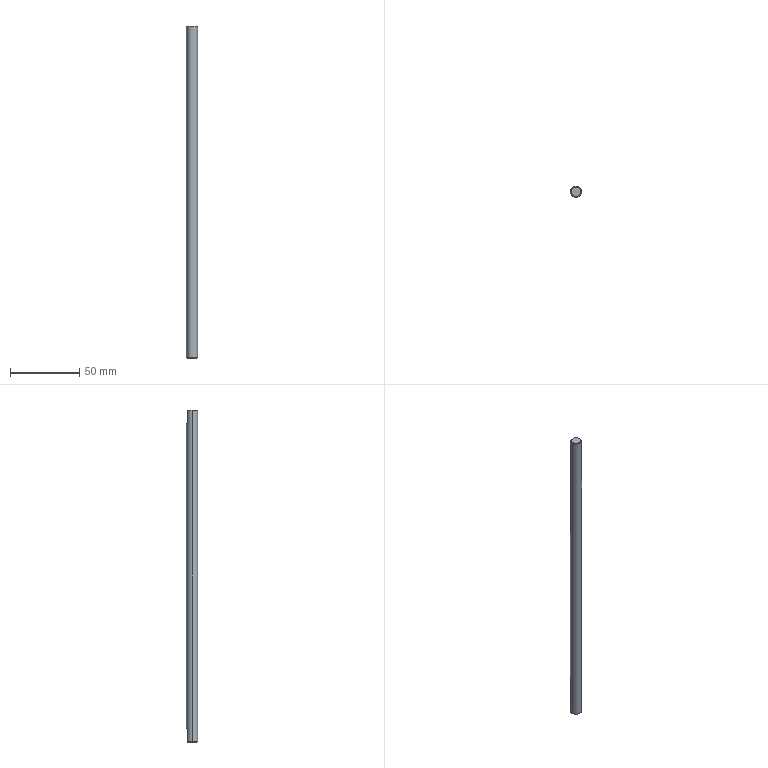Part | STEP file | CA-10-012Pusher Rod_Default | 1 solid | 14 faces | box 8 x 8 x 240 mm | volume 11986 mm3 | cone 6 | plane 6 | cylinder 2 | commonest cylinder face diameters 8 x2
STEP:
#1=CARTESIAN_POINT('',(0.,0.,0.));
#2=DIRECTION('',(0.,0.,1.));
#3=DIRECTION('',(1.,0.,0.));
#4=AXIS2_PLACEMENT_3D('',#1,#2,#3);
#5=CARTESIAN_POINT('',(3.5,0.,120.));
#6=VERTEX_POINT('',#5);
#7=CARTESIAN_POINT('',(1.803,3.,120.));
#8=VERTEX_POINT('',#7);
#9=CARTESIAN_POINT('',(0.,0.,120.));
#10=DIRECTION('',(0.,0.,1.));
#11=DIRECTION('',(1.,0.,0.));
#12=AXIS2_PLACEMENT_3D('',#9,#10,#11);
#13=CIRCLE('',#12,3.5);
#14=CARTESIAN_POINT('',(0.,0.,120.));
#15=DIRECTION('',(0.,0.,-1.));
#16=DIRECTION('',(-1.,0.,0.));
#17=AXIS2_PLACEMENT_3D('',#14,#15,#16);
#18=CONICAL_SURFACE('',#17,3.5,0.7854);
#19=CARTESIAN_POINT('',(3.142,0.));
#20=DIRECTION('',(-1.,0.));
#21=VECTOR('',#20,1.);
#22=LINE('',#19,#21);
#23=(GEOMETRIC_REPRESENTATION_CONTEXT(2)PARAMETRIC_REPRESENTATION_CONTEXT()REPRESENTATION_CONTEXT('',''));
#24=DEFINITIONAL_REPRESENTATION('',(#22),#23);
#25=PCURVE('',#18,#24);
#26=CARTESIAN_POINT('',(0.,0.,120.));
#27=DIRECTION('',(0.,0.,1.));
#28=DIRECTION('',(1.,0.,0.));
#29=AXIS2_PLACEMENT_3D('',#26,#27,#28);
#30=PLANE('',#29);
#31=CARTESIAN_POINT('',(0.,0.));
#32=DIRECTION('',(1.,0.));
#33=AXIS2_PLACEMENT_2D('',#31,#32);
#34=CIRCLE('',#33,3.5);
#35=(GEOMETRIC_REPRESENTATION_CONTEXT(2)PARAMETRIC_REPRESENTATION_CONTEXT()REPRESENTATION_CONTEXT('',''));
#36=DEFINITIONAL_REPRESENTATION('',(#34),#35);
#37=PCURVE('',#30,#36);
#38=SURFACE_CURVE('',#13,(#25,#37),.PCURVE_S1.);
#39=EDGE_CURVE('',#6,#8,#38,.T.);
#40=ORIENTED_EDGE('',*,*,#39,.F.);
#41=CARTESIAN_POINT('',(4.,0.,119.5));
#42=VERTEX_POINT('',#41);
#43=CARTESIAN_POINT('',(3.5,0.,120.));
#44=DIRECTION('',(0.7071,0.,-0.7071));
#45=VECTOR('',#44,1.);
#46=LINE('',#43,#45);
#47=CARTESIAN_POINT('',(3.142,0.));
#48=DIRECTION('',(0.,1.));
#49=VECTOR('',#48,1.);
#50=LINE('',#47,#49);
#51=(GEOMETRIC_REPRESENTATION_CONTEXT(2)PARAMETRIC_REPRESENTATION_CONTEXT()REPRESENTATION_CONTEXT('',''));
#52=DEFINITIONAL_REPRESENTATION('',(#50),#51);
#53=PCURVE('',#18,#52);
#54=CARTESIAN_POINT('',(0.,0.,120.));
#55=DIRECTION('',(0.,0.,-1.));
#56=DIRECTION('',(-1.,0.,0.));
#57=AXIS2_PLACEMENT_3D('',#54,#55,#56);
#58=CONICAL_SURFACE('',#57,3.5,0.7854);
#59=CARTESIAN_POINT('',(3.142,0.));
#60=DIRECTION('',(0.,1.));
#61=VECTOR('',#60,1.);
#62=LINE('',#59,#61);
#63=(GEOMETRIC_REPRESENTATION_CONTEXT(2)PARAMETRIC_REPRESENTATION_CONTEXT()REPRESENTATION_CONTEXT('',''));
#64=DEFINITIONAL_REPRESENTATION('',(#62),#63);
#65=PCURVE('',#58,#64);
#66=SURFACE_CURVE('',#46,(#53,#65),.PCURVE_S1.);
#67=EDGE_CURVE('',#6,#42,#66,.T.);
#68=ORIENTED_EDGE('',*,*,#67,.T.);
#69=CARTESIAN_POINT('',(2.646,3.,119.5));
#70=VERTEX_POINT('',#69);
#71=CARTESIAN_POINT('',(0.,0.,119.5));
#72=DIRECTION('',(0.,0.,-1.));
#73=DIRECTION('',(1.,0.,0.));
#74=AXIS2_PLACEMENT_3D('',#71,#72,#73);
#75=CIRCLE('',#74,4.);
#76=CARTESIAN_POINT('',(-3.142,0.5));
#77=DIRECTION('',(1.,0.));
#78=VECTOR('',#77,1.);
#79=LINE('',#76,#78);
#80=(GEOMETRIC_REPRESENTATION_CONTEXT(2)PARAMETRIC_REPRESENTATION_CONTEXT()REPRESENTATION_CONTEXT('',''));
#81=DEFINITIONAL_REPRESENTATION('',(#79),#80);
#82=PCURVE('',#18,#81);
#83=CARTESIAN_POINT('',(0.,0.,120.));
#84=DIRECTION('',(0.,0.,-1.));
#85=DIRECTION('',(-1.,0.,0.));
#86=AXIS2_PLACEMENT_3D('',#83,#84,#85);
#87=CYLINDRICAL_SURFACE('',#86,4.);
#88=CARTESIAN_POINT('',(-3.142,0.5));
#89=DIRECTION('',(1.,0.));
#90=VECTOR('',#89,1.);
#91=LINE('',#88,#90);
#92=(GEOMETRIC_REPRESENTATION_CONTEXT(2)PARAMETRIC_REPRESENTATION_CONTEXT()REPRESENTATION_CONTEXT('',''));
#93=DEFINITIONAL_REPRESENTATION('',(#91),#92);
#94=PCURVE('',#87,#93);
#95=SURFACE_CURVE('',#75,(#82,#94),.PCURVE_S1.);
#96=EDGE_CURVE('',#70,#42,#95,.T.);
#97=ORIENTED_EDGE('',*,*,#96,.F.);
#98=CARTESIAN_POINT('',(1.803,3.,120.));
#99=CARTESIAN_POINT('',(2.092,3.,119.851));
#100=CARTESIAN_POINT('',(2.373,3.,119.68));
#101=CARTESIAN_POINT('',(2.646,3.,119.5));
#102=B_SPLINE_CURVE_WITH_KNOTS('',3,(#98,#99,#100,#101),.UNSPECIFIED.,.F.,.F.,(4,4),(0.01215,0.01312),.PIECEWISE_BEZIER_KNOTS.);
#103=CARTESIAN_POINT('',(2.112,0.));
#104=CARTESIAN_POINT('',(2.115,0.006781));
#105=CARTESIAN_POINT('',(2.122,0.02043));
#106=CARTESIAN_POINT('',(2.131,0.04117));
#107=CARTESIAN_POINT('',(2.14,0.06217));
#108=CARTESIAN_POINT('',(2.15,0.08341));
#109=CARTESIAN_POINT('',(2.159,0.1049));
#110=CARTESIAN_POINT('',(2.167,0.1266));
#111=CARTESIAN_POINT('',(2.176,0.1485));
#112=CARTESIAN_POINT('',(2.185,0.1707));
#113=CARTESIAN_POINT('',(2.194,0.1931));
#114=CARTESIAN_POINT('',(2.202,0.2156));
#115=CARTESIAN_POINT('',(2.21,0.2384));
#116=CARTESIAN_POINT('',(2.218,0.2614));
#117=CARTESIAN_POINT('',(2.226,0.2845));
#118=CARTESIAN_POINT('',(2.234,0.3078));
#119=CARTESIAN_POINT('',(2.242,0.3313));
#120=CARTESIAN_POINT('',(2.25,0.355));
#121=CARTESIAN_POINT('',(2.257,0.3788));
#122=CARTESIAN_POINT('',(2.265,0.4028));
#123=CARTESIAN_POINT('',(2.272,0.4269));
#124=CARTESIAN_POINT('',(2.279,0.4511));
#125=CARTESIAN_POINT('',(2.287,0.4755));
#126=CARTESIAN_POINT('',(2.291,0.4918));
#127=CARTESIAN_POINT('',(2.294,0.5));
#128=B_SPLINE_CURVE_WITH_KNOTS('',3,(#103,#104,#105,#106,#107,#108,#109,#110,#111,#112,#113,#114,#115,#116,#117,#118,#119,#120,#121,#122,#123,#124,#125,#126,#127),.UNSPECIFIED.,.F.,.F.,(4,1,1,1,1,1,1,1,1,1,1,1,1,1,1,1,1,1,1,1,1,1,4),(0.01215,0.01219,0.01223,0.01228,0.01232,0.01237,0.01241,0.01245,0.0125,0.01254,0.01259,0.01263,0.01268,0.01272,0.01276,0.01281,0.01285,0.0129,0.01294,0.01299,0.01303,0.01307,0.01312),.QUASI_UNIFORM_KNOTS.);
#129=(GEOMETRIC_REPRESENTATION_CONTEXT(2)PARAMETRIC_REPRESENTATION_CONTEXT()REPRESENTATION_CONTEXT('',''));
#130=DEFINITIONAL_REPRESENTATION('',(#128),#129);
#131=PCURVE('',#18,#130);
#132=CARTESIAN_POINT('',(-3.991,3.,110.));
#133=DIRECTION('',(0.,-1.,0.));
#134=DIRECTION('',(0.,0.,-1.));
#135=AXIS2_PLACEMENT_3D('',#132,#133,#134);
#136=PLANE('',#135);
#137=CARTESIAN_POINT('',(-10.,5.794));
#138=CARTESIAN_POINT('',(-9.851,6.084));
#139=CARTESIAN_POINT('',(-9.68,6.365));
#140=CARTESIAN_POINT('',(-9.5,6.637));
#141=B_SPLINE_CURVE_WITH_KNOTS('',3,(#137,#138,#139,#140),.UNSPECIFIED.,.F.,.F.,(4,4),(0.01215,0.01312),.PIECEWISE_BEZIER_KNOTS.);
#142=(GEOMETRIC_REPRESENTATION_CONTEXT(2)PARAMETRIC_REPRESENTATION_CONTEXT()REPRESENTATION_CONTEXT('',''));
#143=DEFINITIONAL_REPRESENTATION('',(#141),#142);
#144=PCURVE('',#136,#143);
#145=SURFACE_CURVE('',#102,(#131,#144),.PCURVE_S1.);
#146=EDGE_CURVE('',#8,#70,#145,.T.);
#147=ORIENTED_EDGE('',*,*,#146,.F.);
#148=EDGE_LOOP('',(#40,#68,#97,#147));
#149=FACE_BOUND('',#148,.T.);
#150=ADVANCED_FACE('',(#149),#18,.T.);
#151=ORIENTED_EDGE('',*,*,#67,.F.);
#152=CARTESIAN_POINT('',(-3.5,0.,120.));
#153=VERTEX_POINT('',#152);
#154=CARTESIAN_POINT('',(0.,0.,120.));
#155=DIRECTION('',(0.,0.,1.));
#156=DIRECTION('',(1.,0.,0.));
#157=AXIS2_PLACEMENT_3D('',#154,#155,#156);
#158=CIRCLE('',#157,3.5);
#159=CARTESIAN_POINT('',(9.425,0.));
#160=DIRECTION('',(-1.,0.));
#161=VECTOR('',#160,1.);
#162=LINE('',#159,#161);
#163=(GEOMETRIC_REPRESENTATION_CONTEXT(2)PARAMETRIC_REPRESENTATION_CONTEXT()REPRESENTATION_CONTEXT('',''));
#164=DEFINITIONAL_REPRESENTATION('',(#162),#163);
#165=PCURVE('',#58,#164);
#166=CARTESIAN_POINT('',(0.,0.));
#167=DIRECTION('',(1.,0.));
#168=AXIS2_PLACEMENT_2D('',#166,#167);
#169=CIRCLE('',#168,3.5);
#170=(GEOMETRIC_REPRESENTATION_CONTEXT(2)PARAMETRIC_REPRESENTATION_CONTEXT()REPRESENTATION_CONTEXT('',''));
#171=DEFINITIONAL_REPRESENTATION('',(#169),#170);
#172=PCURVE('',#30,#171);
#173=SURFACE_CURVE('',#158,(#165,#172),.PCURVE_S1.);
#174=EDGE_CURVE('',#153,#6,#173,.T.);
#175=ORIENTED_EDGE('',*,*,#174,.F.);
#176=CARTESIAN_POINT('',(-4.,0.,119.5));
#177=VERTEX_POINT('',#176);
#178=CARTESIAN_POINT('',(-3.5,0.,120.));
#179=DIRECTION('',(-0.7071,0.,-0.7071));
#180=VECTOR('',#179,1.);
#181=LINE('',#178,#180);
#182=CARTESIAN_POINT('',(6.283,0.));
#183=DIRECTION('',(0.,1.));
#184=VECTOR('',#183,1.);
#185=LINE('',#182,#184);
#186=(GEOMETRIC_REPRESENTATION_CONTEXT(2)PARAMETRIC_REPRESENTATION_CONTEXT()REPRESENTATION_CONTEXT('',''));
#187=DEFINITIONAL_REPRESENTATION('',(#185),#186);
#188=PCURVE('',#58,#187);
#189=CARTESIAN_POINT('',(0.,0.,120.));
#190=DIRECTION('',(0.,0.,-1.));
#191=DIRECTION('',(-1.,0.,0.));
#192=AXIS2_PLACEMENT_3D('',#189,#190,#191);
#193=CONICAL_SURFACE('',#192,3.5,0.7854);
#194=CARTESIAN_POINT('',(0.,0.));
#195=DIRECTION('',(0.,1.));
#196=VECTOR('',#195,1.);
#197=LINE('',#194,#196);
#198=(GEOMETRIC_REPRESENTATION_CONTEXT(2)PARAMETRIC_REPRESENTATION_CONTEXT()REPRESENTATION_CONTEXT('',''));
#199=DEFINITIONAL_REPRESENTATION('',(#197),#198);
#200=PCURVE('',#193,#199);
#201=SURFACE_CURVE('',#181,(#188,#200),.PCURVE_S1.);
#202=EDGE_CURVE('',#153,#177,#201,.T.);
#203=ORIENTED_EDGE('',*,*,#202,.T.);
#204=CARTESIAN_POINT('',(0.,0.,119.5));
#205=DIRECTION('',(0.,0.,-1.));
#206=DIRECTION('',(1.,0.,0.));
#207=AXIS2_PLACEMENT_3D('',#204,#205,#206);
#208=CIRCLE('',#207,4.);
#209=CARTESIAN_POINT('',(3.142,0.5));
#210=DIRECTION('',(1.,0.));
#211=VECTOR('',#210,1.);
#212=LINE('',#209,#211);
#213=(GEOMETRIC_REPRESENTATION_CONTEXT(2)PARAMETRIC_REPRESENTATION_CONTEXT()REPRESENTATION_CONTEXT('',''));
#214=DEFINITIONAL_REPRESENTATION('',(#212),#213);
#215=PCURVE('',#58,#214);
#216=CARTESIAN_POINT('',(0.,0.,120.));
#217=DIRECTION('',(0.,0.,-1.));
#218=DIRECTION('',(-1.,0.,0.));
#219=AXIS2_PLACEMENT_3D('',#216,#217,#218);
#220=CYLINDRICAL_SURFACE('',#219,4.);
#221=CARTESIAN_POINT('',(3.142,0.5));
#222=DIRECTION('',(1.,0.));
#223=VECTOR('',#222,1.);
#224=LINE('',#221,#223);
#225=(GEOMETRIC_REPRESENTATION_CONTEXT(2)PARAMETRIC_REPRESENTATION_CONTEXT()REPRESENTATION_CONTEXT('',''));
#226=DEFINITIONAL_REPRESENTATION('',(#224),#225);
#227=PCURVE('',#220,#226);
#228=SURFACE_CURVE('',#208,(#215,#227),.PCURVE_S1.);
#229=EDGE_CURVE('',#42,#177,#228,.T.);
#230=ORIENTED_EDGE('',*,*,#229,.F.);
#231=EDGE_LOOP('',(#151,#175,#203,#230));
#232=FACE_BOUND('',#231,.T.);
#233=ADVANCED_FACE('',(#232),#58,.T.);
#234=CARTESIAN_POINT('',(-3.5,0.,-120.));
#235=VERTEX_POINT('',#234);
#236=CARTESIAN_POINT('',(-1.803,3.,-120.));
#237=VERTEX_POINT('',#236);
#238=CARTESIAN_POINT('',(0.,0.,-120.));
#239=DIRECTION('',(0.,0.,-1.));
#240=DIRECTION('',(1.,0.,0.));
#241=AXIS2_PLACEMENT_3D('',#238,#239,#240);
#242=CIRCLE('',#241,3.5);
#243=CARTESIAN_POINT('',(0.,0.,-119.5));
#244=DIRECTION('',(0.,0.,1.));
#245=DIRECTION('',(1.,0.,0.));
#246=AXIS2_PLACEMENT_3D('',#243,#244,#245);
#247=CONICAL_SURFACE('',#246,4.,0.7854);
#248=CARTESIAN_POINT('',(6.283,-0.5));
#249=DIRECTION('',(-1.,0.));
#250=VECTOR('',#249,1.);
#251=LINE('',#248,#250);
#252=(GEOMETRIC_REPRESENTATION_CONTEXT(2)PARAMETRIC_REPRESENTATION_CONTEXT()REPRESENTATION_CONTEXT('',''));
#253=DEFINITIONAL_REPRESENTATION('',(#251),#252);
#254=PCURVE('',#247,#253);
#255=CARTESIAN_POINT('',(0.,0.,-120.));
#256=DIRECTION('',(0.,0.,1.));
#257=DIRECTION('',(1.,0.,0.));
#258=AXIS2_PLACEMENT_3D('',#255,#256,#257);
#259=PLANE('',#258);
#260=CARTESIAN_POINT('',(3.5,0.));
#261=CARTESIAN_POINT('',(3.5,-6.062));
#262=CARTESIAN_POINT('',(-1.75,-3.031));
#263=CARTESIAN_POINT('',(-7.,0.));
#264=CARTESIAN_POINT('',(-1.75,3.031));
#265=CARTESIAN_POINT('',(3.5,6.062));
#266=CARTESIAN_POINT('',(3.5,0.));
#267=(BOUNDED_CURVE()B_SPLINE_CURVE(2,(#260,#261,#262,#263,#264,#265,#266),.UNSPECIFIED.,.T.,.F.)B_SPLINE_CURVE_WITH_KNOTS((1,2,2,2,2,1),(-2.094,0.,2.094,4.189,6.283,8.378),.UNSPECIFIED.)CURVE()GEOMETRIC_REPRESENTATION_ITEM()RATIONAL_B_SPLINE_CURVE((1.,0.5,1.,0.5,1.,0.5,1.))REPRESENTATION_ITEM(''));
#268=(GEOMETRIC_REPRESENTATION_CONTEXT(2)PARAMETRIC_REPRESENTATION_CONTEXT()REPRESENTATION_CONTEXT('',''));
#269=DEFINITIONAL_REPRESENTATION('',(#267),#268);
#270=PCURVE('',#259,#269);
#271=SURFACE_CURVE('',#242,(#254,#270),.PCURVE_S1.);
#272=EDGE_CURVE('',#235,#237,#271,.T.);
#273=ORIENTED_EDGE('',*,*,#272,.F.);
#274=CARTESIAN_POINT('',(-4.,0.,-119.5));
#275=VERTEX_POINT('',#274);
#276=CARTESIAN_POINT('',(-4.,0.,-119.5));
#277=DIRECTION('',(-0.7071,0.,0.7071));
#278=VECTOR('',#277,1.);
#279=LINE('',#276,#278);
#280=CARTESIAN_POINT('',(3.142,0.));
#281=DIRECTION('',(0.,1.));
#282=VECTOR('',#281,1.);
#283=LINE('',#280,#282);
#284=(GEOMETRIC_REPRESENTATION_CONTEXT(2)PARAMETRIC_REPRESENTATION_CONTEXT()REPRESENTATION_CONTEXT('',''));
#285=DEFINITIONAL_REPRESENTATION('',(#283),#284);
#286=PCURVE('',#247,#285);
#287=CARTESIAN_POINT('',(0.,0.,-119.5));
#288=DIRECTION('',(0.,0.,1.));
#289=DIRECTION('',(1.,0.,0.));
#290=AXIS2_PLACEMENT_3D('',#287,#288,#289);
#291=CONICAL_SURFACE('',#290,4.,0.7854);
#292=CARTESIAN_POINT('',(3.142,0.));
#293=DIRECTION('',(0.,1.));
#294=VECTOR('',#293,1.);
#295=LINE('',#292,#294);
#296=(GEOMETRIC_REPRESENTATION_CONTEXT(2)PARAMETRIC_REPRESENTATION_CONTEXT()REPRESENTATION_CONTEXT('',''));
#297=DEFINITIONAL_REPRESENTATION('',(#295),#296);
#298=PCURVE('',#291,#297);
#299=SURFACE_CURVE('',#279,(#286,#298),.PCURVE_S1.);
#300=EDGE_CURVE('',#235,#275,#299,.T.);
#301=ORIENTED_EDGE('',*,*,#300,.T.);
#302=CARTESIAN_POINT('',(-2.646,3.,-119.5));
#303=VERTEX_POINT('',#302);
#304=CARTESIAN_POINT('',(0.,0.,-119.5));
#305=DIRECTION('',(0.,0.,1.));
#306=DIRECTION('',(1.,0.,0.));
#307=AXIS2_PLACEMENT_3D('',#304,#305,#306);
#308=CIRCLE('',#307,4.);
#309=CARTESIAN_POINT('',(0.,0.));
#310=DIRECTION('',(1.,0.));
#311=VECTOR('',#310,1.);
#312=LINE('',#309,#311);
#313=(GEOMETRIC_REPRESENTATION_CONTEXT(2)PARAMETRIC_REPRESENTATION_CONTEXT()REPRESENTATION_CONTEXT('',''));
#314=DEFINITIONAL_REPRESENTATION('',(#312),#313);
#315=PCURVE('',#247,#314);
#316=CARTESIAN_POINT('',(3.142,239.5));
#317=DIRECTION('',(-1.,0.));
#318=VECTOR('',#317,1.);
#319=LINE('',#316,#318);
#320=(GEOMETRIC_REPRESENTATION_CONTEXT(2)PARAMETRIC_REPRESENTATION_CONTEXT()REPRESENTATION_CONTEXT('',''));
#321=DEFINITIONAL_REPRESENTATION('',(#319),#320);
#322=PCURVE('',#87,#321);
#323=SURFACE_CURVE('',#308,(#315,#322),.PCURVE_S1.);
#324=EDGE_CURVE('',#303,#275,#323,.T.);
#325=ORIENTED_EDGE('',*,*,#324,.F.);
#326=CARTESIAN_POINT('',(-2.646,3.,-119.5));
#327=CARTESIAN_POINT('',(-2.374,3.,-119.68));
#328=CARTESIAN_POINT('',(-2.095,3.,-119.849));
#329=CARTESIAN_POINT('',(-1.803,3.,-120.));
#330=B_SPLINE_CURVE_WITH_KNOTS('',3,(#326,#327,#328,#329),.UNSPECIFIED.,.F.,.F.,(4,4),(0.007417,0.008397),.PIECEWISE_BEZIER_KNOTS.);
#331=CARTESIAN_POINT('',(2.294,0.));
#332=CARTESIAN_POINT('',(2.291,-0.008169));
#333=CARTESIAN_POINT('',(2.287,-0.02446));
#334=CARTESIAN_POINT('',(2.279,-0.04877));
#335=CARTESIAN_POINT('',(2.272,-0.07295));
#336=CARTESIAN_POINT('',(2.265,-0.09698));
#337=CARTESIAN_POINT('',(2.257,-0.1209));
#338=CARTESIAN_POINT('',(2.25,-0.1446));
#339=CARTESIAN_POINT('',(2.242,-0.1682));
#340=CARTESIAN_POINT('',(2.235,-0.1916));
#341=CARTESIAN_POINT('',(2.227,-0.2149));
#342=CARTESIAN_POINT('',(2.219,-0.238));
#343=CARTESIAN_POINT('',(2.21,-0.2609));
#344=CARTESIAN_POINT('',(2.202,-0.2836));
#345=CARTESIAN_POINT('',(2.194,-0.3062));
#346=CARTESIAN_POINT('',(2.185,-0.3285));
#347=CARTESIAN_POINT('',(2.177,-0.3507));
#348=CARTESIAN_POINT('',(2.168,-0.3727));
#349=CARTESIAN_POINT('',(2.159,-0.3945));
#350=CARTESIAN_POINT('',(2.15,-0.416));
#351=CARTESIAN_POINT('',(2.141,-0.4374));
#352=CARTESIAN_POINT('',(2.131,-0.4585));
#353=CARTESIAN_POINT('',(2.122,-0.4794));
#354=CARTESIAN_POINT('',(2.115,-0.4932));
#355=CARTESIAN_POINT('',(2.112,-0.5));
#356=B_SPLINE_CURVE_WITH_KNOTS('',3,(#331,#332,#333,#334,#335,#336,#337,#338,#339,#340,#341,#342,#343,#344,#345,#346,#347,#348,#349,#350,#351,#352,#353,#354,#355),.UNSPECIFIED.,.F.,.F.,(4,1,1,1,1,1,1,1,1,1,1,1,1,1,1,1,1,1,1,1,1,1,4),(0.007417,0.007461,0.007506,0.007551,0.007595,0.00764,0.007684,0.007729,0.007773,0.007818,0.007863,0.007907,0.007952,0.007996,0.008041,0.008085,0.00813,0.008175,0.008219,0.008264,0.008308,0.008353,0.008397),.QUASI_UNIFORM_KNOTS.);
#357=(GEOMETRIC_REPRESENTATION_CONTEXT(2)PARAMETRIC_REPRESENTATION_CONTEXT()REPRESENTATION_CONTEXT('',''));
#358=DEFINITIONAL_REPRESENTATION('',(#356),#357);
#359=PCURVE('',#247,#358);
#360=CARTESIAN_POINT('',(-3.991,3.,-110.));
#361=DIRECTION('',(0.,1.,0.));
#362=DIRECTION('',(0.,0.,1.));
#363=AXIS2_PLACEMENT_3D('',#360,#361,#362);
#364=PLANE('',#363);
#365=CARTESIAN_POINT('',(-9.5,1.346));
#366=CARTESIAN_POINT('',(-9.68,1.617));
#367=CARTESIAN_POINT('',(-9.849,1.896));
#368=CARTESIAN_POINT('',(-10.,2.189));
#369=B_SPLINE_CURVE_WITH_KNOTS('',3,(#365,#366,#367,#368),.UNSPECIFIED.,.F.,.F.,(4,4),(0.007417,0.008397),.PIECEWISE_BEZIER_KNOTS.);
#370=(GEOMETRIC_REPRESENTATION_CONTEXT(2)PARAMETRIC_REPRESENTATION_CONTEXT()REPRESENTATION_CONTEXT('',''));
#371=DEFINITIONAL_REPRESENTATION('',(#369),#370);
#372=PCURVE('',#364,#371);
#373=SURFACE_CURVE('',#330,(#359,#372),.PCURVE_S1.);
#374=EDGE_CURVE('',#303,#237,#373,.T.);
#375=ORIENTED_EDGE('',*,*,#374,.T.);
#376=EDGE_LOOP('',(#273,#301,#325,#375));
#377=FACE_BOUND('',#376,.T.);
#378=ADVANCED_FACE('',(#377),#247,.T.);
#379=ORIENTED_EDGE('',*,*,#300,.F.);
#380=CARTESIAN_POINT('',(3.5,0.,-120.));
#381=VERTEX_POINT('',#380);
#382=CARTESIAN_POINT('',(0.,0.,-120.));
#383=DIRECTION('',(0.,0.,-1.));
#384=DIRECTION('',(1.,0.,0.));
#385=AXIS2_PLACEMENT_3D('',#382,#383,#384);
#386=CIRCLE('',#385,3.5);
#387=CARTESIAN_POINT('',(6.283,-0.5));
#388=DIRECTION('',(-1.,0.));
#389=VECTOR('',#388,1.);
#390=LINE('',#387,#389);
#391=(GEOMETRIC_REPRESENTATION_CONTEXT(2)PARAMETRIC_REPRESENTATION_CONTEXT()REPRESENTATION_CONTEXT('',''));
#392=DEFINITIONAL_REPRESENTATION('',(#390),#391);
#393=PCURVE('',#291,#392);
#394=CARTESIAN_POINT('',(3.5,0.));
#395=CARTESIAN_POINT('',(3.5,-6.062));
#396=CARTESIAN_POINT('',(-1.75,-3.031));
#397=CARTESIAN_POINT('',(-7.,0.));
#398=CARTESIAN_POINT('',(-1.75,3.031));
#399=CARTESIAN_POINT('',(3.5,6.062));
#400=CARTESIAN_POINT('',(3.5,0.));
#401=(BOUNDED_CURVE()B_SPLINE_CURVE(2,(#394,#395,#396,#397,#398,#399,#400),.UNSPECIFIED.,.T.,.F.)B_SPLINE_CURVE_WITH_KNOTS((1,2,2,2,2,1),(-2.094,0.,2.094,4.189,6.283,8.378),.UNSPECIFIED.)CURVE()GEOMETRIC_REPRESENTATION_ITEM()RATIONAL_B_SPLINE_CURVE((1.,0.5,1.,0.5,1.,0.5,1.))REPRESENTATION_ITEM(''));
#402=(GEOMETRIC_REPRESENTATION_CONTEXT(2)PARAMETRIC_REPRESENTATION_CONTEXT()REPRESENTATION_CONTEXT('',''));
#403=DEFINITIONAL_REPRESENTATION('',(#401),#402);
#404=PCURVE('',#259,#403);
#405=SURFACE_CURVE('',#386,(#393,#404),.PCURVE_S1.);
#406=EDGE_CURVE('',#381,#235,#405,.T.);
#407=ORIENTED_EDGE('',*,*,#406,.F.);
#408=CARTESIAN_POINT('',(4.,0.,-119.5));
#409=VERTEX_POINT('',#408);
#410=CARTESIAN_POINT('',(4.,0.,-119.5));
#411=DIRECTION('',(0.7071,0.,0.7071));
#412=VECTOR('',#411,1.);
#413=LINE('',#410,#412);
#414=CARTESIAN_POINT('',(6.283,0.));
#415=DIRECTION('',(0.,1.));
#416=VECTOR('',#415,1.);
#417=LINE('',#414,#416);
#418=(GEOMETRIC_REPRESENTATION_CONTEXT(2)PARAMETRIC_REPRESENTATION_CONTEXT()REPRESENTATION_CONTEXT('',''));
#419=DEFINITIONAL_REPRESENTATION('',(#417),#418);
#420=PCURVE('',#291,#419);
#421=CARTESIAN_POINT('',(0.,0.,-119.5));
#422=DIRECTION('',(0.,0.,1.));
#423=DIRECTION('',(1.,0.,0.));
#424=AXIS2_PLACEMENT_3D('',#421,#422,#423);
#425=CONICAL_SURFACE('',#424,4.,0.7854);
#426=CARTESIAN_POINT('',(0.,0.));
#427=DIRECTION('',(0.,1.));
#428=VECTOR('',#427,1.);
#429=LINE('',#426,#428);
#430=(GEOMETRIC_REPRESENTATION_CONTEXT(2)PARAMETRIC_REPRESENTATION_CONTEXT()REPRESENTATION_CONTEXT('',''));
#431=DEFINITIONAL_REPRESENTATION('',(#429),#430);
#432=PCURVE('',#425,#431);
#433=SURFACE_CURVE('',#413,(#420,#432),.PCURVE_S1.);
#434=EDGE_CURVE('',#381,#409,#433,.T.);
#435=ORIENTED_EDGE('',*,*,#434,.T.);
#436=CARTESIAN_POINT('',(0.,0.,-119.5));
#437=DIRECTION('',(0.,0.,1.));
#438=DIRECTION('',(1.,0.,0.));
#439=AXIS2_PLACEMENT_3D('',#436,#437,#438);
#440=CIRCLE('',#439,4.);
#441=CARTESIAN_POINT('',(0.,0.));
#442=DIRECTION('',(1.,0.));
#443=VECTOR('',#442,1.);
#444=LINE('',#441,#443);
#445=(GEOMETRIC_REPRESENTATION_CONTEXT(2)PARAMETRIC_REPRESENTATION_CONTEXT()REPRESENTATION_CONTEXT('',''));
#446=DEFINITIONAL_REPRESENTATION('',(#444),#445);
#447=PCURVE('',#291,#446);
#448=CARTESIAN_POINT('',(9.425,239.5));
#449=DIRECTION('',(-1.,0.));
#450=VECTOR('',#449,1.);
#451=LINE('',#448,#450);
#452=(GEOMETRIC_REPRESENTATION_CONTEXT(2)PARAMETRIC_REPRESENTATION_CONTEXT()REPRESENTATION_CONTEXT('',''));
#453=DEFINITIONAL_REPRESENTATION('',(#451),#452);
#454=PCURVE('',#220,#453);
#455=SURFACE_CURVE('',#440,(#447,#454),.PCURVE_S1.);
#456=EDGE_CURVE('',#275,#409,#455,.T.);
#457=ORIENTED_EDGE('',*,*,#456,.F.);
#458=EDGE_LOOP('',(#379,#407,#435,#457));
#459=FACE_BOUND('',#458,.T.);
#460=ADVANCED_FACE('',(#459),#291,.T.);
#461=ORIENTED_EDGE('',*,*,#96,.T.);
#462=CARTESIAN_POINT('',(4.,0.,120.));
#463=DIRECTION('',(0.,0.,-1.));
#464=VECTOR('',#463,1.);
#465=LINE('',#462,#464);
#466=CARTESIAN_POINT('',(3.142,0.));
#467=DIRECTION('',(0.,1.));
#468=VECTOR('',#467,1.);
#469=LINE('',#466,#468);
#470=(GEOMETRIC_REPRESENTATION_CONTEXT(2)PARAMETRIC_REPRESENTATION_CONTEXT()REPRESENTATION_CONTEXT('',''));
#471=DEFINITIONAL_REPRESENTATION('',(#469),#470);
#472=PCURVE('',#87,#471);
#473=CARTESIAN_POINT('',(3.142,0.));
#474=DIRECTION('',(0.,1.));
#475=VECTOR('',#474,1.);
#476=LINE('',#473,#475);
#477=(GEOMETRIC_REPRESENTATION_CONTEXT(2)PARAMETRIC_REPRESENTATION_CONTEXT()REPRESENTATION_CONTEXT('',''));
#478=DEFINITIONAL_REPRESENTATION('',(#476),#477);
#479=PCURVE('',#220,#478);
#480=SURFACE_CURVE('',#465,(#472,#479),.PCURVE_S1.);
#481=EDGE_CURVE('',#42,#409,#480,.T.);
#482=ORIENTED_EDGE('',*,*,#481,.T.);
#483=CARTESIAN_POINT('',(2.646,3.,-119.5));
#484=VERTEX_POINT('',#483);
#485=CARTESIAN_POINT('',(0.,0.,-119.5));
#486=DIRECTION('',(0.,0.,1.));
#487=DIRECTION('',(1.,0.,0.));
#488=AXIS2_PLACEMENT_3D('',#485,#486,#487);
#489=CIRCLE('',#488,4.);
#490=CARTESIAN_POINT('',(3.142,239.5));
#491=DIRECTION('',(-1.,0.));
#492=VECTOR('',#491,1.);
#493=LINE('',#490,#492);
#494=(GEOMETRIC_REPRESENTATION_CONTEXT(2)PARAMETRIC_REPRESENTATION_CONTEXT()REPRESENTATION_CONTEXT('',''));
#495=DEFINITIONAL_REPRESENTATION('',(#493),#494);
#496=PCURVE('',#87,#495);
#497=CARTESIAN_POINT('',(0.,0.));
#498=DIRECTION('',(1.,0.));
#499=VECTOR('',#498,1.);
#500=LINE('',#497,#499);
#501=(GEOMETRIC_REPRESENTATION_CONTEXT(2)PARAMETRIC_REPRESENTATION_CONTEXT()REPRESENTATION_CONTEXT('',''));
#502=DEFINITIONAL_REPRESENTATION('',(#500),#501);
#503=PCURVE('',#425,#502);
#504=SURFACE_CURVE('',#489,(#496,#503),.PCURVE_S1.);
#505=EDGE_CURVE('',#409,#484,#504,.T.);
#506=ORIENTED_EDGE('',*,*,#505,.T.);
#507=CARTESIAN_POINT('',(2.646,3.,-110.));
#508=VERTEX_POINT('',#507);
#509=CARTESIAN_POINT('',(2.646,3.,120.));
#510=DIRECTION('',(0.,0.,-1.));
#511=VECTOR('',#510,1.);
#512=LINE('',#509,#511);
#513=CARTESIAN_POINT('',(2.294,0.));
#514=DIRECTION('',(0.,1.));
#515=VECTOR('',#514,1.);
#516=LINE('',#513,#515);
#517=(GEOMETRIC_REPRESENTATION_CONTEXT(2)PARAMETRIC_REPRESENTATION_CONTEXT()REPRESENTATION_CONTEXT('',''));
#518=DEFINITIONAL_REPRESENTATION('',(#516),#517);
#519=PCURVE('',#87,#518);
#520=CARTESIAN_POINT('',(230.,6.637));
#521=DIRECTION('',(-1.,0.));
#522=VECTOR('',#521,1.);
#523=LINE('',#520,#522);
#524=(GEOMETRIC_REPRESENTATION_CONTEXT(2)PARAMETRIC_REPRESENTATION_CONTEXT()REPRESENTATION_CONTEXT('',''));
#525=DEFINITIONAL_REPRESENTATION('',(#523),#524);
#526=PCURVE('',#364,#525);
#527=SURFACE_CURVE('',#512,(#519,#526),.PCURVE_S1.);
#528=EDGE_CURVE('',#508,#484,#527,.T.);
#529=ORIENTED_EDGE('',*,*,#528,.F.);
#530=CARTESIAN_POINT('',(-2.646,3.,-110.));
#531=VERTEX_POINT('',#530);
#532=CARTESIAN_POINT('',(0.,0.,-110.));
#533=DIRECTION('',(0.,0.,-1.));
#534=DIRECTION('',(-1.,0.,0.));
#535=AXIS2_PLACEMENT_3D('',#532,#533,#534);
#536=CIRCLE('',#535,4.);
#537=CARTESIAN_POINT('',(0.,230.));
#538=DIRECTION('',(1.,0.));
#539=VECTOR('',#538,1.);
#540=LINE('',#537,#539);
#541=(GEOMETRIC_REPRESENTATION_CONTEXT(2)PARAMETRIC_REPRESENTATION_CONTEXT()REPRESENTATION_CONTEXT('',''));
#542=DEFINITIONAL_REPRESENTATION('',(#540),#541);
#543=PCURVE('',#87,#542);
#544=CARTESIAN_POINT('',(0.,0.,-110.));
#545=DIRECTION('',(0.,0.,-1.));
#546=DIRECTION('',(1.,0.,0.));
#547=AXIS2_PLACEMENT_3D('',#544,#545,#546);
#548=PLANE('',#547);
#549=CARTESIAN_POINT('',(0.,0.));
#550=DIRECTION('',(-1.,0.));
#551=AXIS2_PLACEMENT_2D('',#549,#550);
#552=CIRCLE('',#551,4.);
#553=(GEOMETRIC_REPRESENTATION_CONTEXT(2)PARAMETRIC_REPRESENTATION_CONTEXT()REPRESENTATION_CONTEXT('',''));
#554=DEFINITIONAL_REPRESENTATION('',(#552),#553);
#555=PCURVE('',#548,#554);
#556=SURFACE_CURVE('',#536,(#543,#555),.PCURVE_S1.);
#557=EDGE_CURVE('',#531,#508,#556,.T.);
#558=ORIENTED_EDGE('',*,*,#557,.F.);
#559=CARTESIAN_POINT('',(-2.646,3.,120.));
#560=DIRECTION('',(0.,0.,1.));
#561=VECTOR('',#560,1.);
#562=LINE('',#559,#561);
#563=CARTESIAN_POINT('',(0.8481,0.));
#564=DIRECTION('',(0.,-1.));
#565=VECTOR('',#564,1.);
#566=LINE('',#563,#565);
#567=(GEOMETRIC_REPRESENTATION_CONTEXT(2)PARAMETRIC_REPRESENTATION_CONTEXT()REPRESENTATION_CONTEXT('',''));
#568=DEFINITIONAL_REPRESENTATION('',(#566),#567);
#569=PCURVE('',#87,#568);
#570=CARTESIAN_POINT('',(230.,1.346));
#571=DIRECTION('',(1.,0.));
#572=VECTOR('',#571,1.);
#573=LINE('',#570,#572);
#574=(GEOMETRIC_REPRESENTATION_CONTEXT(2)PARAMETRIC_REPRESENTATION_CONTEXT()REPRESENTATION_CONTEXT('',''));
#575=DEFINITIONAL_REPRESENTATION('',(#573),#574);
#576=PCURVE('',#364,#575);
#577=SURFACE_CURVE('',#562,(#569,#576),.PCURVE_S1.);
#578=EDGE_CURVE('',#303,#531,#577,.T.);
#579=ORIENTED_EDGE('',*,*,#578,.F.);
#580=ORIENTED_EDGE('',*,*,#324,.T.);
#581=CARTESIAN_POINT('',(-4.,0.,120.));
#582=DIRECTION('',(0.,0.,-1.));
#583=VECTOR('',#582,1.);
#584=LINE('',#581,#583);
#585=CARTESIAN_POINT('',(0.,0.));
#586=DIRECTION('',(0.,1.));
#587=VECTOR('',#586,1.);
#588=LINE('',#585,#587);
#589=(GEOMETRIC_REPRESENTATION_CONTEXT(2)PARAMETRIC_REPRESENTATION_CONTEXT()REPRESENTATION_CONTEXT('',''));
#590=DEFINITIONAL_REPRESENTATION('',(#588),#589);
#591=PCURVE('',#87,#590);
#592=CARTESIAN_POINT('',(6.283,0.));
#593=DIRECTION('',(0.,1.));
#594=VECTOR('',#593,1.);
#595=LINE('',#592,#594);
#596=(GEOMETRIC_REPRESENTATION_CONTEXT(2)PARAMETRIC_REPRESENTATION_CONTEXT()REPRESENTATION_CONTEXT('',''));
#597=DEFINITIONAL_REPRESENTATION('',(#595),#596);
#598=PCURVE('',#220,#597);
#599=SURFACE_CURVE('',#584,(#591,#598),.PCURVE_S1.);
#600=EDGE_CURVE('',#177,#275,#599,.T.);
#601=ORIENTED_EDGE('',*,*,#600,.F.);
#602=CARTESIAN_POINT('',(-2.646,3.,119.5));
#603=VERTEX_POINT('',#602);
#604=CARTESIAN_POINT('',(0.,0.,119.5));
#605=DIRECTION('',(0.,0.,-1.));
#606=DIRECTION('',(1.,0.,0.));
#607=AXIS2_PLACEMENT_3D('',#604,#605,#606);
#608=CIRCLE('',#607,4.);
#609=CARTESIAN_POINT('',(-3.142,0.5));
#610=DIRECTION('',(1.,0.));
#611=VECTOR('',#610,1.);
#612=LINE('',#609,#611);
#613=(GEOMETRIC_REPRESENTATION_CONTEXT(2)PARAMETRIC_REPRESENTATION_CONTEXT()REPRESENTATION_CONTEXT('',''));
#614=DEFINITIONAL_REPRESENTATION('',(#612),#613);
#615=PCURVE('',#87,#614);
#616=CARTESIAN_POINT('',(-3.142,0.5));
#617=DIRECTION('',(1.,0.));
#618=VECTOR('',#617,1.);
#619=LINE('',#616,#618);
#620=(GEOMETRIC_REPRESENTATION_CONTEXT(2)PARAMETRIC_REPRESENTATION_CONTEXT()REPRESENTATION_CONTEXT('',''));
#621=DEFINITIONAL_REPRESENTATION('',(#619),#620);
#622=PCURVE('',#193,#621);
#623=SURFACE_CURVE('',#608,(#615,#622),.PCURVE_S1.);
#624=EDGE_CURVE('',#177,#603,#623,.T.);
#625=ORIENTED_EDGE('',*,*,#624,.T.);
#626=CARTESIAN_POINT('',(-2.646,3.,110.));
#627=VERTEX_POINT('',#626);
#628=CARTESIAN_POINT('',(-2.646,3.,120.));
#629=DIRECTION('',(0.,0.,-1.));
#630=VECTOR('',#629,1.);
#631=LINE('',#628,#630);
#632=CARTESIAN_POINT('',(0.8481,0.));
#633=DIRECTION('',(0.,1.));
#634=VECTOR('',#633,1.);
#635=LINE('',#632,#634);
#636=(GEOMETRIC_REPRESENTATION_CONTEXT(2)PARAMETRIC_REPRESENTATION_CONTEXT()REPRESENTATION_CONTEXT('',''));
#637=DEFINITIONAL_REPRESENTATION('',(#635),#636);
#638=PCURVE('',#87,#637);
#639=CARTESIAN_POINT('',(-10.,1.346));
#640=DIRECTION('',(1.,0.));
#641=VECTOR('',#640,1.);
#642=LINE('',#639,#641);
#643=(GEOMETRIC_REPRESENTATION_CONTEXT(2)PARAMETRIC_REPRESENTATION_CONTEXT()REPRESENTATION_CONTEXT('',''));
#644=DEFINITIONAL_REPRESENTATION('',(#642),#643);
#645=PCURVE('',#136,#644);
#646=SURFACE_CURVE('',#631,(#638,#645),.PCURVE_S1.);
#647=EDGE_CURVE('',#603,#627,#646,.T.);
#648=ORIENTED_EDGE('',*,*,#647,.T.);
#649=CARTESIAN_POINT('',(2.646,3.,110.));
#650=VERTEX_POINT('',#649);
#651=CARTESIAN_POINT('',(0.,0.,110.));
#652=DIRECTION('',(0.,0.,1.));
#653=DIRECTION('',(1.,0.,0.));
#654=AXIS2_PLACEMENT_3D('',#651,#652,#653);
#655=CIRCLE('',#654,4.);
#656=CARTESIAN_POINT('',(3.142,10.));
#657=DIRECTION('',(-1.,0.));
#658=VECTOR('',#657,1.);
#659=LINE('',#656,#658);
#660=(GEOMETRIC_REPRESENTATION_CONTEXT(2)PARAMETRIC_REPRESENTATION_CONTEXT()REPRESENTATION_CONTEXT('',''));
#661=DEFINITIONAL_REPRESENTATION('',(#659),#660);
#662=PCURVE('',#87,#661);
#663=CARTESIAN_POINT('',(0.,0.,110.));
#664=DIRECTION('',(0.,0.,1.));
#665=DIRECTION('',(1.,0.,0.));
#666=AXIS2_PLACEMENT_3D('',#663,#664,#665);
#667=PLANE('',#666);
#668=CARTESIAN_POINT('',(0.,0.));
#669=DIRECTION('',(1.,0.));
#670=AXIS2_PLACEMENT_2D('',#668,#669);
#671=CIRCLE('',#670,4.);
#672=(GEOMETRIC_REPRESENTATION_CONTEXT(2)PARAMETRIC_REPRESENTATION_CONTEXT()REPRESENTATION_CONTEXT('',''));
#673=DEFINITIONAL_REPRESENTATION('',(#671),#672);
#674=PCURVE('',#667,#673);
#675=SURFACE_CURVE('',#655,(#662,#674),.PCURVE_S1.);
#676=EDGE_CURVE('',#650,#627,#675,.T.);
#677=ORIENTED_EDGE('',*,*,#676,.F.);
#678=CARTESIAN_POINT('',(2.646,3.,120.));
#679=DIRECTION('',(0.,0.,1.));
#680=VECTOR('',#679,1.);
#681=LINE('',#678,#680);
#682=CARTESIAN_POINT('',(2.294,0.));
#683=DIRECTION('',(0.,-1.));
#684=VECTOR('',#683,1.);
#685=LINE('',#682,#684);
#686=(GEOMETRIC_REPRESENTATION_CONTEXT(2)PARAMETRIC_REPRESENTATION_CONTEXT()REPRESENTATION_CONTEXT('',''));
#687=DEFINITIONAL_REPRESENTATION('',(#685),#686);
#688=PCURVE('',#87,#687);
#689=CARTESIAN_POINT('',(-10.,6.637));
#690=DIRECTION('',(-1.,0.));
#691=VECTOR('',#690,1.);
#692=LINE('',#689,#691);
#693=(GEOMETRIC_REPRESENTATION_CONTEXT(2)PARAMETRIC_REPRESENTATION_CONTEXT()REPRESENTATION_CONTEXT('',''));
#694=DEFINITIONAL_REPRESENTATION('',(#692),#693);
#695=PCURVE('',#136,#694);
#696=SURFACE_CURVE('',#681,(#688,#695),.PCURVE_S1.);
#697=EDGE_CURVE('',#650,#70,#696,.T.);
#698=ORIENTED_EDGE('',*,*,#697,.T.);
#699=EDGE_LOOP('',(#461,#482,#506,#529,#558,#579,#580,#601,#625,#648,#677,#698));
#700=FACE_BOUND('',#699,.T.);
#701=ADVANCED_FACE('',(#700),#87,.T.);
#702=ORIENTED_EDGE('',*,*,#481,.F.);
#703=ORIENTED_EDGE('',*,*,#229,.T.);
#704=ORIENTED_EDGE('',*,*,#600,.T.);
#705=ORIENTED_EDGE('',*,*,#456,.T.);
#706=EDGE_LOOP('',(#702,#703,#704,#705));
#707=FACE_BOUND('',#706,.T.);
#708=ADVANCED_FACE('',(#707),#220,.T.);
#709=CARTESIAN_POINT('',(1.803,3.,-120.));
#710=VERTEX_POINT('',#709);
#711=CARTESIAN_POINT('',(-3.991,3.,-120.));
#712=DIRECTION('',(1.,0.,0.));
#713=VECTOR('',#712,1.);
#714=LINE('',#711,#713);
#715=CARTESIAN_POINT('',(-3.991,3.));
#716=DIRECTION('',(1.,0.));
#717=VECTOR('',#716,1.);
#718=LINE('',#715,#717);
#719=(GEOMETRIC_REPRESENTATION_CONTEXT(2)PARAMETRIC_REPRESENTATION_CONTEXT()REPRESENTATION_CONTEXT('',''));
#720=DEFINITIONAL_REPRESENTATION('',(#718),#719);
#721=PCURVE('',#259,#720);
#722=CARTESIAN_POINT('',(-10.,0.));
#723=DIRECTION('',(0.,1.));
#724=VECTOR('',#723,1.);
#725=LINE('',#722,#724);
#726=(GEOMETRIC_REPRESENTATION_CONTEXT(2)PARAMETRIC_REPRESENTATION_CONTEXT()REPRESENTATION_CONTEXT('',''));
#727=DEFINITIONAL_REPRESENTATION('',(#725),#726);
#728=PCURVE('',#364,#727);
#729=SURFACE_CURVE('',#714,(#721,#728),.PCURVE_S1.);
#730=EDGE_CURVE('',#237,#710,#729,.T.);
#731=ORIENTED_EDGE('',*,*,#730,.T.);
#732=CARTESIAN_POINT('',(0.,0.,-120.));
#733=DIRECTION('',(0.,0.,-1.));
#734=DIRECTION('',(1.,0.,0.));
#735=AXIS2_PLACEMENT_3D('',#732,#733,#734);
#736=CIRCLE('',#735,3.5);
#737=CARTESIAN_POINT('',(3.5,0.));
#738=CARTESIAN_POINT('',(3.5,-6.062));
#739=CARTESIAN_POINT('',(-1.75,-3.031));
#740=CARTESIAN_POINT('',(-7.,0.));
#741=CARTESIAN_POINT('',(-1.75,3.031));
#742=CARTESIAN_POINT('',(3.5,6.062));
#743=CARTESIAN_POINT('',(3.5,0.));
#744=(BOUNDED_CURVE()B_SPLINE_CURVE(2,(#737,#738,#739,#740,#741,#742,#743),.UNSPECIFIED.,.T.,.F.)B_SPLINE_CURVE_WITH_KNOTS((1,2,2,2,2,1),(-2.094,0.,2.094,4.189,6.283,8.378),.UNSPECIFIED.)CURVE()GEOMETRIC_REPRESENTATION_ITEM()RATIONAL_B_SPLINE_CURVE((1.,0.5,1.,0.5,1.,0.5,1.))REPRESENTATION_ITEM(''));
#745=(GEOMETRIC_REPRESENTATION_CONTEXT(2)PARAMETRIC_REPRESENTATION_CONTEXT()REPRESENTATION_CONTEXT('',''));
#746=DEFINITIONAL_REPRESENTATION('',(#744),#745);
#747=PCURVE('',#259,#746);
#748=CARTESIAN_POINT('',(6.283,-0.5));
#749=DIRECTION('',(-1.,0.));
#750=VECTOR('',#749,1.);
#751=LINE('',#748,#750);
#752=(GEOMETRIC_REPRESENTATION_CONTEXT(2)PARAMETRIC_REPRESENTATION_CONTEXT()REPRESENTATION_CONTEXT('',''));
#753=DEFINITIONAL_REPRESENTATION('',(#751),#752);
#754=PCURVE('',#425,#753);
#755=SURFACE_CURVE('',#736,(#747,#754),.PCURVE_S1.);
#756=EDGE_CURVE('',#710,#381,#755,.T.);
#757=ORIENTED_EDGE('',*,*,#756,.T.);
#758=ORIENTED_EDGE('',*,*,#406,.T.);
#759=ORIENTED_EDGE('',*,*,#272,.T.);
#760=EDGE_LOOP('',(#731,#757,#758,#759));
#761=FACE_BOUND('',#760,.T.);
#762=ADVANCED_FACE('',(#761),#259,.F.);
#763=ORIENTED_EDGE('',*,*,#434,.F.);
#764=ORIENTED_EDGE('',*,*,#756,.F.);
#765=CARTESIAN_POINT('',(1.803,3.,-120.));
#766=CARTESIAN_POINT('',(2.092,3.,-119.851));
#767=CARTESIAN_POINT('',(2.373,3.,-119.68));
#768=CARTESIAN_POINT('',(2.646,3.,-119.5));
#769=B_SPLINE_CURVE_WITH_KNOTS('',3,(#765,#766,#767,#768),.UNSPECIFIED.,.F.,.F.,(4,4),(0.01215,0.01312),.PIECEWISE_BEZIER_KNOTS.);
#770=CARTESIAN_POINT('',(1.03,-0.5));
#771=CARTESIAN_POINT('',(1.026,-0.4932));
#772=CARTESIAN_POINT('',(1.02,-0.4796));
#773=CARTESIAN_POINT('',(1.011,-0.4588));
#774=CARTESIAN_POINT('',(1.001,-0.4378));
#775=CARTESIAN_POINT('',(0.9921,-0.4166));
#776=CARTESIAN_POINT('',(0.983,-0.3951));
#777=CARTESIAN_POINT('',(0.9741,-0.3734));
#778=CARTESIAN_POINT('',(0.9653,-0.3515));
#779=CARTESIAN_POINT('',(0.9566,-0.3293));
#780=CARTESIAN_POINT('',(0.9481,-0.3069));
#781=CARTESIAN_POINT('',(0.9397,-0.2844));
#782=CARTESIAN_POINT('',(0.9314,-0.2616));
#783=CARTESIAN_POINT('',(0.9232,-0.2386));
#784=CARTESIAN_POINT('',(0.9152,-0.2155));
#785=CARTESIAN_POINT('',(0.9073,-0.1922));
#786=CARTESIAN_POINT('',(0.8995,-0.1687));
#787=CARTESIAN_POINT('',(0.8918,-0.145));
#788=CARTESIAN_POINT('',(0.8842,-0.1212));
#789=CARTESIAN_POINT('',(0.8768,-0.09725));
#790=CARTESIAN_POINT('',(0.8694,-0.07314));
#791=CARTESIAN_POINT('',(0.8622,-0.0489));
#792=CARTESIAN_POINT('',(0.8551,-0.02452));
#793=CARTESIAN_POINT('',(0.8504,-0.008187));
#794=CARTESIAN_POINT('',(0.8481,0.));
#795=B_SPLINE_CURVE_WITH_KNOTS('',3,(#770,#771,#772,#773,#774,#775,#776,#777,#778,#779,#780,#781,#782,#783,#784,#785,#786,#787,#788,#789,#790,#791,#792,#793,#794),.UNSPECIFIED.,.F.,.F.,(4,1,1,1,1,1,1,1,1,1,1,1,1,1,1,1,1,1,1,1,1,1,4),(0.01215,0.01219,0.01223,0.01228,0.01232,0.01237,0.01241,0.01245,0.0125,0.01254,0.01259,0.01263,0.01268,0.01272,0.01276,0.01281,0.01285,0.0129,0.01294,0.01299,0.01303,0.01307,0.01312),.QUASI_UNIFORM_KNOTS.);
#796=(GEOMETRIC_REPRESENTATION_CONTEXT(2)PARAMETRIC_REPRESENTATION_CONTEXT()REPRESENTATION_CONTEXT('',''));
#797=DEFINITIONAL_REPRESENTATION('',(#795),#796);
#798=PCURVE('',#425,#797);
#799=CARTESIAN_POINT('',(-10.,5.794));
#800=CARTESIAN_POINT('',(-9.851,6.084));
#801=CARTESIAN_POINT('',(-9.68,6.365));
#802=CARTESIAN_POINT('',(-9.5,6.637));
#803=B_SPLINE_CURVE_WITH_KNOTS('',3,(#799,#800,#801,#802),.UNSPECIFIED.,.F.,.F.,(4,4),(0.01215,0.01312),.PIECEWISE_BEZIER_KNOTS.);
#804=(GEOMETRIC_REPRESENTATION_CONTEXT(2)PARAMETRIC_REPRESENTATION_CONTEXT()REPRESENTATION_CONTEXT('',''));
#805=DEFINITIONAL_REPRESENTATION('',(#803),#804);
#806=PCURVE('',#364,#805);
#807=SURFACE_CURVE('',#769,(#798,#806),.PCURVE_S1.);
#808=EDGE_CURVE('',#710,#484,#807,.T.);
#809=ORIENTED_EDGE('',*,*,#808,.T.);
#810=ORIENTED_EDGE('',*,*,#505,.F.);
#811=EDGE_LOOP('',(#763,#764,#809,#810));
#812=FACE_BOUND('',#811,.T.);
#813=ADVANCED_FACE('',(#812),#425,.T.);
#814=CARTESIAN_POINT('',(-1.803,3.,120.));
#815=VERTEX_POINT('',#814);
#816=CARTESIAN_POINT('',(-3.991,3.,120.));
#817=DIRECTION('',(1.,0.,0.));
#818=VECTOR('',#817,1.);
#819=LINE('',#816,#818);
#820=CARTESIAN_POINT('',(-3.991,3.));
#821=DIRECTION('',(1.,0.));
#822=VECTOR('',#821,1.);
#823=LINE('',#820,#822);
#824=(GEOMETRIC_REPRESENTATION_CONTEXT(2)PARAMETRIC_REPRESENTATION_CONTEXT()REPRESENTATION_CONTEXT('',''));
#825=DEFINITIONAL_REPRESENTATION('',(#823),#824);
#826=PCURVE('',#30,#825);
#827=CARTESIAN_POINT('',(-10.,0.));
#828=DIRECTION('',(0.,1.));
#829=VECTOR('',#828,1.);
#830=LINE('',#827,#829);
#831=(GEOMETRIC_REPRESENTATION_CONTEXT(2)PARAMETRIC_REPRESENTATION_CONTEXT()REPRESENTATION_CONTEXT('',''));
#832=DEFINITIONAL_REPRESENTATION('',(#830),#831);
#833=PCURVE('',#136,#832);
#834=SURFACE_CURVE('',#819,(#826,#833),.PCURVE_S1.);
#835=EDGE_CURVE('',#815,#8,#834,.T.);
#836=ORIENTED_EDGE('',*,*,#835,.F.);
#837=CARTESIAN_POINT('',(0.,0.,120.));
#838=DIRECTION('',(0.,0.,1.));
#839=DIRECTION('',(1.,0.,0.));
#840=AXIS2_PLACEMENT_3D('',#837,#838,#839);
#841=CIRCLE('',#840,3.5);
#842=CARTESIAN_POINT('',(0.,0.));
#843=DIRECTION('',(1.,0.));
#844=AXIS2_PLACEMENT_2D('',#842,#843);
#845=CIRCLE('',#844,3.5);
#846=(GEOMETRIC_REPRESENTATION_CONTEXT(2)PARAMETRIC_REPRESENTATION_CONTEXT()REPRESENTATION_CONTEXT('',''));
#847=DEFINITIONAL_REPRESENTATION('',(#845),#846);
#848=PCURVE('',#30,#847);
#849=CARTESIAN_POINT('',(3.142,0.));
#850=DIRECTION('',(-1.,0.));
#851=VECTOR('',#850,1.);
#852=LINE('',#849,#851);
#853=(GEOMETRIC_REPRESENTATION_CONTEXT(2)PARAMETRIC_REPRESENTATION_CONTEXT()REPRESENTATION_CONTEXT('',''));
#854=DEFINITIONAL_REPRESENTATION('',(#852),#853);
#855=PCURVE('',#193,#854);
#856=SURFACE_CURVE('',#841,(#848,#855),.PCURVE_S1.);
#857=EDGE_CURVE('',#815,#153,#856,.T.);
#858=ORIENTED_EDGE('',*,*,#857,.T.);
#859=ORIENTED_EDGE('',*,*,#174,.T.);
#860=ORIENTED_EDGE('',*,*,#39,.T.);
#861=EDGE_LOOP('',(#836,#858,#859,#860));
#862=FACE_BOUND('',#861,.T.);
#863=ADVANCED_FACE('',(#862),#30,.T.);
#864=ORIENTED_EDGE('',*,*,#202,.F.);
#865=ORIENTED_EDGE('',*,*,#857,.F.);
#866=CARTESIAN_POINT('',(-2.646,3.,119.5));
#867=CARTESIAN_POINT('',(-2.374,3.,119.68));
#868=CARTESIAN_POINT('',(-2.095,3.,119.849));
#869=CARTESIAN_POINT('',(-1.803,3.,120.));
#870=B_SPLINE_CURVE_WITH_KNOTS('',3,(#866,#867,#868,#869),.UNSPECIFIED.,.F.,.F.,(4,4),(0.007417,0.008397),.PIECEWISE_BEZIER_KNOTS.);
#871=CARTESIAN_POINT('',(0.8481,0.5));
#872=CARTESIAN_POINT('',(0.8504,0.4918));
#873=CARTESIAN_POINT('',(0.855,0.4755));
#874=CARTESIAN_POINT('',(0.8621,0.4512));
#875=CARTESIAN_POINT('',(0.8694,0.4271));
#876=CARTESIAN_POINT('',(0.8767,0.403));
#877=CARTESIAN_POINT('',(0.8841,0.3791));
#878=CARTESIAN_POINT('',(0.8916,0.3554));
#879=CARTESIAN_POINT('',(0.8993,0.3318));
#880=CARTESIAN_POINT('',(0.9071,0.3084));
#881=CARTESIAN_POINT('',(0.915,0.2851));
#882=CARTESIAN_POINT('',(0.923,0.262));
#883=CARTESIAN_POINT('',(0.9311,0.2391));
#884=CARTESIAN_POINT('',(0.9394,0.2164));
#885=CARTESIAN_POINT('',(0.9478,0.1938));
#886=CARTESIAN_POINT('',(0.9563,0.1715));
#887=CARTESIAN_POINT('',(0.965,0.1493));
#888=CARTESIAN_POINT('',(0.9738,0.1273));
#889=CARTESIAN_POINT('',(0.9827,0.1055));
#890=CARTESIAN_POINT('',(0.9918,0.08398));
#891=CARTESIAN_POINT('',(1.001,0.06263));
#892=CARTESIAN_POINT('',(1.01,0.04151));
#893=CARTESIAN_POINT('',(1.02,0.02062));
#894=CARTESIAN_POINT('',(1.026,0.006846));
#895=CARTESIAN_POINT('',(1.03,0.));
#896=B_SPLINE_CURVE_WITH_KNOTS('',3,(#871,#872,#873,#874,#875,#876,#877,#878,#879,#880,#881,#882,#883,#884,#885,#886,#887,#888,#889,#890,#891,#892,#893,#894,#895),.UNSPECIFIED.,.F.,.F.,(4,1,1,1,1,1,1,1,1,1,1,1,1,1,1,1,1,1,1,1,1,1,4),(0.007417,0.007461,0.007506,0.007551,0.007595,0.00764,0.007684,0.007729,0.007773,0.007818,0.007863,0.007907,0.007952,0.007996,0.008041,0.008085,0.00813,0.008175,0.008219,0.008264,0.008308,0.008353,0.008397),.QUASI_UNIFORM_KNOTS.);
#897=(GEOMETRIC_REPRESENTATION_CONTEXT(2)PARAMETRIC_REPRESENTATION_CONTEXT()REPRESENTATION_CONTEXT('',''));
#898=DEFINITIONAL_REPRESENTATION('',(#896),#897);
#899=PCURVE('',#193,#898);
#900=CARTESIAN_POINT('',(-9.5,1.346));
#901=CARTESIAN_POINT('',(-9.68,1.617));
#902=CARTESIAN_POINT('',(-9.849,1.896));
#903=CARTESIAN_POINT('',(-10.,2.189));
#904=B_SPLINE_CURVE_WITH_KNOTS('',3,(#900,#901,#902,#903),.UNSPECIFIED.,.F.,.F.,(4,4),(0.007417,0.008397),.PIECEWISE_BEZIER_KNOTS.);
#905=(GEOMETRIC_REPRESENTATION_CONTEXT(2)PARAMETRIC_REPRESENTATION_CONTEXT()REPRESENTATION_CONTEXT('',''));
#906=DEFINITIONAL_REPRESENTATION('',(#904),#905);
#907=PCURVE('',#136,#906);
#908=SURFACE_CURVE('',#870,(#899,#907),.PCURVE_S1.);
#909=EDGE_CURVE('',#603,#815,#908,.T.);
#910=ORIENTED_EDGE('',*,*,#909,.F.);
#911=ORIENTED_EDGE('',*,*,#624,.F.);
#912=EDGE_LOOP('',(#864,#865,#910,#911));
#913=FACE_BOUND('',#912,.T.);
#914=ADVANCED_FACE('',(#913),#193,.T.);
#915=ORIENTED_EDGE('',*,*,#676,.T.);
#916=CARTESIAN_POINT('',(-3.991,3.,110.));
#917=DIRECTION('',(1.,0.,0.));
#918=VECTOR('',#917,1.);
#919=LINE('',#916,#918);
#920=CARTESIAN_POINT('',(-3.991,3.));
#921=DIRECTION('',(1.,0.));
#922=VECTOR('',#921,1.);
#923=LINE('',#920,#922);
#924=(GEOMETRIC_REPRESENTATION_CONTEXT(2)PARAMETRIC_REPRESENTATION_CONTEXT()REPRESENTATION_CONTEXT('',''));
#925=DEFINITIONAL_REPRESENTATION('',(#923),#924);
#926=PCURVE('',#667,#925);
#927=CARTESIAN_POINT('',(0.,0.));
#928=DIRECTION('',(0.,1.));
#929=VECTOR('',#928,1.);
#930=LINE('',#927,#929);
#931=(GEOMETRIC_REPRESENTATION_CONTEXT(2)PARAMETRIC_REPRESENTATION_CONTEXT()REPRESENTATION_CONTEXT('',''));
#932=DEFINITIONAL_REPRESENTATION('',(#930),#931);
#933=PCURVE('',#136,#932);
#934=SURFACE_CURVE('',#919,(#926,#933),.PCURVE_S1.);
#935=EDGE_CURVE('',#627,#650,#934,.T.);
#936=ORIENTED_EDGE('',*,*,#935,.T.);
#937=EDGE_LOOP('',(#915,#936));
#938=FACE_BOUND('',#937,.T.);
#939=ADVANCED_FACE('',(#938),#667,.T.);
#940=ORIENTED_EDGE('',*,*,#909,.T.);
#941=ORIENTED_EDGE('',*,*,#835,.T.);
#942=ORIENTED_EDGE('',*,*,#146,.T.);
#943=ORIENTED_EDGE('',*,*,#697,.F.);
#944=ORIENTED_EDGE('',*,*,#935,.F.);
#945=ORIENTED_EDGE('',*,*,#647,.F.);
#946=EDGE_LOOP('',(#940,#941,#942,#943,#944,#945));
#947=FACE_BOUND('',#946,.T.);
#948=ADVANCED_FACE('',(#947),#136,.F.);
#949=ORIENTED_EDGE('',*,*,#557,.T.);
#950=CARTESIAN_POINT('',(-3.991,3.,-110.));
#951=DIRECTION('',(1.,0.,0.));
#952=VECTOR('',#951,1.);
#953=LINE('',#950,#952);
#954=CARTESIAN_POINT('',(-3.991,-3.));
#955=DIRECTION('',(1.,0.));
#956=VECTOR('',#955,1.);
#957=LINE('',#954,#956);
#958=(GEOMETRIC_REPRESENTATION_CONTEXT(2)PARAMETRIC_REPRESENTATION_CONTEXT()REPRESENTATION_CONTEXT('',''));
#959=DEFINITIONAL_REPRESENTATION('',(#957),#958);
#960=PCURVE('',#548,#959);
#961=CARTESIAN_POINT('',(0.,0.));
#962=DIRECTION('',(0.,1.));
#963=VECTOR('',#962,1.);
#964=LINE('',#961,#963);
#965=(GEOMETRIC_REPRESENTATION_CONTEXT(2)PARAMETRIC_REPRESENTATION_CONTEXT()REPRESENTATION_CONTEXT('',''));
#966=DEFINITIONAL_REPRESENTATION('',(#964),#965);
#967=PCURVE('',#364,#966);
#968=SURFACE_CURVE('',#953,(#960,#967),.PCURVE_S1.);
#969=EDGE_CURVE('',#531,#508,#968,.T.);
#970=ORIENTED_EDGE('',*,*,#969,.F.);
#971=EDGE_LOOP('',(#949,#970));
#972=FACE_BOUND('',#971,.T.);
#973=ADVANCED_FACE('',(#972),#548,.T.);
#974=ORIENTED_EDGE('',*,*,#578,.T.);
#975=ORIENTED_EDGE('',*,*,#969,.T.);
#976=ORIENTED_EDGE('',*,*,#528,.T.);
#977=ORIENTED_EDGE('',*,*,#808,.F.);
#978=ORIENTED_EDGE('',*,*,#730,.F.);
#979=ORIENTED_EDGE('',*,*,#374,.F.);
#980=EDGE_LOOP('',(#974,#975,#976,#977,#978,#979));
#981=FACE_BOUND('',#980,.T.);
#982=ADVANCED_FACE('',(#981),#364,.T.);
#983=CLOSED_SHELL('',(#150,#233,#378,#460,#701,#708,#762,#813,#863,#914,#939,#948,#973,#982));
#984=MANIFOLD_SOLID_BREP('',#983);
#985=(LENGTH_UNIT()NAMED_UNIT(*)SI_UNIT(.MILLI.,.METRE.));
#986=UNCERTAINTY_MEASURE_WITH_UNIT(LENGTH_MEASURE(0.00002),#985,'','');
#987=(NAMED_UNIT(*)PLANE_ANGLE_UNIT()SI_UNIT($,.RADIAN.));
#988=(NAMED_UNIT(*)SI_UNIT($,.STERADIAN.)SOLID_ANGLE_UNIT());
#989=(GEOMETRIC_REPRESENTATION_CONTEXT(3)GLOBAL_UNCERTAINTY_ASSIGNED_CONTEXT((#986))GLOBAL_UNIT_ASSIGNED_CONTEXT((#985,#987,#988))REPRESENTATION_CONTEXT('',''));
#990=ADVANCED_BREP_SHAPE_REPRESENTATION('',(#4,#984),#989);